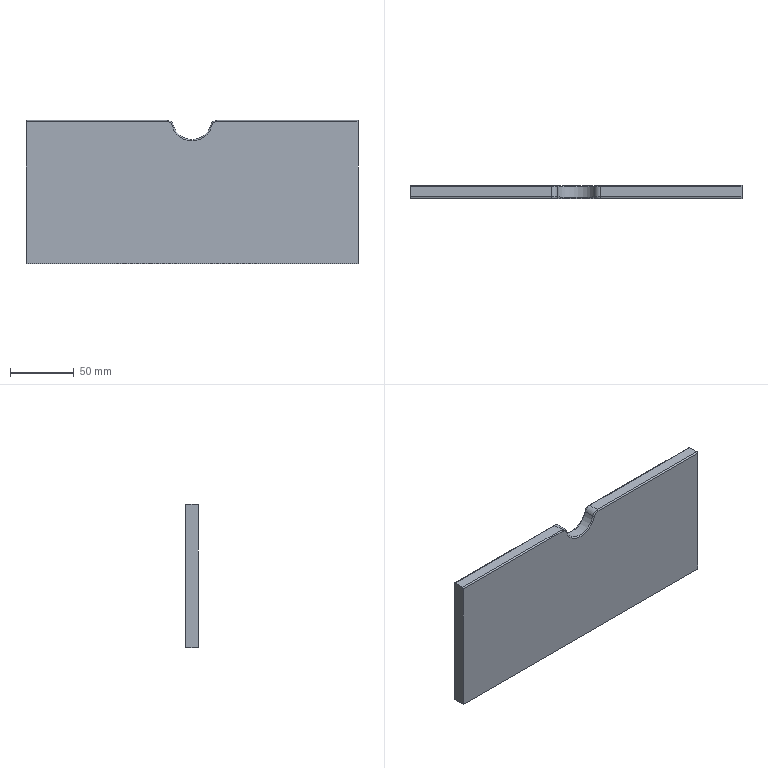Part | STEP file | Drawer | 1 solid | 20 faces | box 260 x 10 x 112 mm | volume 287478 mm3 | plane 7 | cylinder 7 | torus 6 | commonest cylinder face diameters 2 x4 10 x2 30 x1
STEP:
#1=CARTESIAN_POINT('',(0.,0.,0.));
#2=DIRECTION('',(0.,0.,1.));
#3=DIRECTION('',(1.,0.,0.));
#4=AXIS2_PLACEMENT_3D('',#1,#2,#3);
#5=CARTESIAN_POINT('',(-19.365,-9.,112.));
#6=VERTEX_POINT('',#5);
#7=CARTESIAN_POINT('',(-19.365,-1.,112.));
#8=VERTEX_POINT('',#7);
#9=CARTESIAN_POINT('',(-19.365,-10.,112.));
#10=DIRECTION('',(0.,1.,0.));
#11=VECTOR('',#10,1.);
#12=LINE('',#9,#11);
#13=CARTESIAN_POINT('',(130.,0.,112.));
#14=DIRECTION('',(0.,0.,-1.));
#15=DIRECTION('',(-1.,0.,0.));
#16=AXIS2_PLACEMENT_3D('',#13,#14,#15);
#17=PLANE('',#16);
#18=CARTESIAN_POINT('',(149.365,-10.));
#19=DIRECTION('',(0.,1.));
#20=VECTOR('',#19,1.);
#21=LINE('',#18,#20);
#22=(GEOMETRIC_REPRESENTATION_CONTEXT(2)PARAMETRIC_REPRESENTATION_CONTEXT()REPRESENTATION_CONTEXT('',''));
#23=DEFINITIONAL_REPRESENTATION('',(#21),#22);
#24=PCURVE('',#17,#23);
#25=CARTESIAN_POINT('',(-19.365,-10.,107.));
#26=DIRECTION('',(0.,1.,0.));
#27=DIRECTION('',(0.,0.,1.));
#28=AXIS2_PLACEMENT_3D('',#25,#26,#27);
#29=CYLINDRICAL_SURFACE('',#28,5.);
#30=CARTESIAN_POINT('',(0.,0.));
#31=DIRECTION('',(0.,1.));
#32=VECTOR('',#31,1.);
#33=LINE('',#30,#32);
#34=(GEOMETRIC_REPRESENTATION_CONTEXT(2)PARAMETRIC_REPRESENTATION_CONTEXT()REPRESENTATION_CONTEXT('',''));
#35=DEFINITIONAL_REPRESENTATION('',(#33),#34);
#36=PCURVE('',#29,#35);
#37=SURFACE_CURVE('',#12,(#24,#36),.PCURVE_S1.);
#38=EDGE_CURVE('',#6,#8,#37,.T.);
#39=ORIENTED_EDGE('',*,*,#38,.F.);
#40=CARTESIAN_POINT('',(-130.,-9.,112.));
#41=VERTEX_POINT('',#40);
#42=CARTESIAN_POINT('',(-130.,-9.,112.));
#43=DIRECTION('',(1.,0.,0.));
#44=VECTOR('',#43,1.);
#45=LINE('',#42,#44);
#46=CARTESIAN_POINT('',(260.,-9.));
#47=DIRECTION('',(-1.,0.));
#48=VECTOR('',#47,1.);
#49=LINE('',#46,#48);
#50=(GEOMETRIC_REPRESENTATION_CONTEXT(2)PARAMETRIC_REPRESENTATION_CONTEXT()REPRESENTATION_CONTEXT('',''));
#51=DEFINITIONAL_REPRESENTATION('',(#49),#50);
#52=PCURVE('',#17,#51);
#53=CARTESIAN_POINT('',(-130.,-9.,111.));
#54=DIRECTION('',(1.,0.,0.));
#55=DIRECTION('',(0.,-1.,0.));
#56=AXIS2_PLACEMENT_3D('',#53,#54,#55);
#57=CYLINDRICAL_SURFACE('',#56,1.);
#58=CARTESIAN_POINT('',(4.712,0.));
#59=DIRECTION('',(0.,1.));
#60=VECTOR('',#59,1.);
#61=LINE('',#58,#60);
#62=(GEOMETRIC_REPRESENTATION_CONTEXT(2)PARAMETRIC_REPRESENTATION_CONTEXT()REPRESENTATION_CONTEXT('',''));
#63=DEFINITIONAL_REPRESENTATION('',(#61),#62);
#64=PCURVE('',#57,#63);
#65=SURFACE_CURVE('',#45,(#52,#64),.PCURVE_S1.);
#66=EDGE_CURVE('',#41,#6,#65,.T.);
#67=ORIENTED_EDGE('',*,*,#66,.F.);
#68=CARTESIAN_POINT('',(-130.,-1.,112.));
#69=VERTEX_POINT('',#68);
#70=CARTESIAN_POINT('',(-130.,0.,112.));
#71=DIRECTION('',(0.,-1.,0.));
#72=VECTOR('',#71,1.);
#73=LINE('',#70,#72);
#74=CARTESIAN_POINT('',(260.,0.));
#75=DIRECTION('',(0.,-1.));
#76=VECTOR('',#75,1.);
#77=LINE('',#74,#76);
#78=(GEOMETRIC_REPRESENTATION_CONTEXT(2)PARAMETRIC_REPRESENTATION_CONTEXT()REPRESENTATION_CONTEXT('',''));
#79=DEFINITIONAL_REPRESENTATION('',(#77),#78);
#80=PCURVE('',#17,#79);
#81=CARTESIAN_POINT('',(-130.,0.,112.));
#82=DIRECTION('',(1.,0.,0.));
#83=DIRECTION('',(0.,0.,-1.));
#84=AXIS2_PLACEMENT_3D('',#81,#82,#83);
#85=PLANE('',#84);
#86=CARTESIAN_POINT('',(0.,0.));
#87=DIRECTION('',(0.,-1.));
#88=VECTOR('',#87,1.);
#89=LINE('',#86,#88);
#90=(GEOMETRIC_REPRESENTATION_CONTEXT(2)PARAMETRIC_REPRESENTATION_CONTEXT()REPRESENTATION_CONTEXT('',''));
#91=DEFINITIONAL_REPRESENTATION('',(#89),#90);
#92=PCURVE('',#85,#91);
#93=SURFACE_CURVE('',#73,(#80,#92),.PCURVE_S1.);
#94=EDGE_CURVE('',#69,#41,#93,.T.);
#95=ORIENTED_EDGE('',*,*,#94,.F.);
#96=CARTESIAN_POINT('',(-130.,-1.,112.));
#97=DIRECTION('',(1.,0.,0.));
#98=VECTOR('',#97,1.);
#99=LINE('',#96,#98);
#100=CARTESIAN_POINT('',(260.,-1.));
#101=DIRECTION('',(-1.,0.));
#102=VECTOR('',#101,1.);
#103=LINE('',#100,#102);
#104=(GEOMETRIC_REPRESENTATION_CONTEXT(2)PARAMETRIC_REPRESENTATION_CONTEXT()REPRESENTATION_CONTEXT('',''));
#105=DEFINITIONAL_REPRESENTATION('',(#103),#104);
#106=PCURVE('',#17,#105);
#107=CARTESIAN_POINT('',(-130.,-1.,111.));
#108=DIRECTION('',(1.,0.,0.));
#109=DIRECTION('',(0.,1.,0.));
#110=AXIS2_PLACEMENT_3D('',#107,#108,#109);
#111=CYLINDRICAL_SURFACE('',#110,1.);
#112=CARTESIAN_POINT('',(1.571,0.));
#113=DIRECTION('',(0.,1.));
#114=VECTOR('',#113,1.);
#115=LINE('',#112,#114);
#116=(GEOMETRIC_REPRESENTATION_CONTEXT(2)PARAMETRIC_REPRESENTATION_CONTEXT()REPRESENTATION_CONTEXT('',''));
#117=DEFINITIONAL_REPRESENTATION('',(#115),#116);
#118=PCURVE('',#111,#117);
#119=SURFACE_CURVE('',#99,(#106,#118),.PCURVE_S1.);
#120=EDGE_CURVE('',#69,#8,#119,.T.);
#121=ORIENTED_EDGE('',*,*,#120,.T.);
#122=EDGE_LOOP('',(#39,#67,#95,#121));
#123=FACE_BOUND('',#122,.F.);
#124=ADVANCED_FACE('',(#123),#17,.F.);
#125=ORIENTED_EDGE('',*,*,#38,.F.);
#126=CARTESIAN_POINT('',(-14.524,-9.,108.25));
#127=VERTEX_POINT('',#126);
#128=CARTESIAN_POINT('',(-19.365,-9.,107.));
#129=DIRECTION('',(0.,1.,0.));
#130=DIRECTION('',(0.,0.,1.));
#131=AXIS2_PLACEMENT_3D('',#128,#129,#130);
#132=CIRCLE('',#131,5.);
#133=CARTESIAN_POINT('',(0.,1.));
#134=DIRECTION('',(1.,0.));
#135=VECTOR('',#134,1.);
#136=LINE('',#133,#135);
#137=(GEOMETRIC_REPRESENTATION_CONTEXT(2)PARAMETRIC_REPRESENTATION_CONTEXT()REPRESENTATION_CONTEXT('',''));
#138=DEFINITIONAL_REPRESENTATION('',(#136),#137);
#139=PCURVE('',#29,#138);
#140=CARTESIAN_POINT('',(-19.365,-9.,107.));
#141=DIRECTION('',(0.,1.,0.));
#142=DIRECTION('',(0.,0.,1.));
#143=AXIS2_PLACEMENT_3D('',#140,#141,#142);
#144=TOROIDAL_SURFACE('',#143,4.,1.);
#145=CARTESIAN_POINT('',(0.,6.283));
#146=DIRECTION('',(1.,0.));
#147=VECTOR('',#146,1.);
#148=LINE('',#145,#147);
#149=(GEOMETRIC_REPRESENTATION_CONTEXT(2)PARAMETRIC_REPRESENTATION_CONTEXT()REPRESENTATION_CONTEXT('',''));
#150=DEFINITIONAL_REPRESENTATION('',(#148),#149);
#151=PCURVE('',#144,#150);
#152=SURFACE_CURVE('',#132,(#139,#151),.PCURVE_S1.);
#153=EDGE_CURVE('',#6,#127,#152,.T.);
#154=ORIENTED_EDGE('',*,*,#153,.T.);
#155=CARTESIAN_POINT('',(-14.524,-1.,108.25));
#156=VERTEX_POINT('',#155);
#157=CARTESIAN_POINT('',(-14.524,-10.,108.25));
#158=DIRECTION('',(0.,1.,0.));
#159=VECTOR('',#158,1.);
#160=LINE('',#157,#159);
#161=CARTESIAN_POINT('',(1.318,0.));
#162=DIRECTION('',(0.,1.));
#163=VECTOR('',#162,1.);
#164=LINE('',#161,#163);
#165=(GEOMETRIC_REPRESENTATION_CONTEXT(2)PARAMETRIC_REPRESENTATION_CONTEXT()REPRESENTATION_CONTEXT('',''));
#166=DEFINITIONAL_REPRESENTATION('',(#164),#165);
#167=PCURVE('',#29,#166);
#168=CARTESIAN_POINT('',(0.,0.,112.));
#169=DIRECTION('',(0.,1.,0.));
#170=DIRECTION('',(1.,0.,0.));
#171=AXIS2_PLACEMENT_3D('',#168,#169,#170);
#172=CYLINDRICAL_SURFACE('',#171,15.);
#173=CARTESIAN_POINT('',(2.889,-10.));
#174=DIRECTION('',(0.,1.));
#175=VECTOR('',#174,1.);
#176=LINE('',#173,#175);
#177=(GEOMETRIC_REPRESENTATION_CONTEXT(2)PARAMETRIC_REPRESENTATION_CONTEXT()REPRESENTATION_CONTEXT('',''));
#178=DEFINITIONAL_REPRESENTATION('',(#176),#177);
#179=PCURVE('',#172,#178);
#180=SURFACE_CURVE('',#160,(#167,#179),.PCURVE_S1.);
#181=EDGE_CURVE('',#127,#156,#180,.T.);
#182=ORIENTED_EDGE('',*,*,#181,.T.);
#183=CARTESIAN_POINT('',(-19.365,-1.,107.));
#184=DIRECTION('',(0.,1.,0.));
#185=DIRECTION('',(0.,0.,1.));
#186=AXIS2_PLACEMENT_3D('',#183,#184,#185);
#187=CIRCLE('',#186,5.);
#188=CARTESIAN_POINT('',(0.,9.));
#189=DIRECTION('',(1.,0.));
#190=VECTOR('',#189,1.);
#191=LINE('',#188,#190);
#192=(GEOMETRIC_REPRESENTATION_CONTEXT(2)PARAMETRIC_REPRESENTATION_CONTEXT()REPRESENTATION_CONTEXT('',''));
#193=DEFINITIONAL_REPRESENTATION('',(#191),#192);
#194=PCURVE('',#29,#193);
#195=CARTESIAN_POINT('',(-19.365,-1.,107.));
#196=DIRECTION('',(0.,-1.,0.));
#197=DIRECTION('',(0.,0.,1.));
#198=AXIS2_PLACEMENT_3D('',#195,#196,#197);
#199=TOROIDAL_SURFACE('',#198,4.,1.);
#200=CARTESIAN_POINT('',(6.283,6.283));
#201=DIRECTION('',(-1.,0.));
#202=VECTOR('',#201,1.);
#203=LINE('',#200,#202);
#204=(GEOMETRIC_REPRESENTATION_CONTEXT(2)PARAMETRIC_REPRESENTATION_CONTEXT()REPRESENTATION_CONTEXT('',''));
#205=DEFINITIONAL_REPRESENTATION('',(#203),#204);
#206=PCURVE('',#199,#205);
#207=SURFACE_CURVE('',#187,(#194,#206),.PCURVE_S1.);
#208=EDGE_CURVE('',#8,#156,#207,.T.);
#209=ORIENTED_EDGE('',*,*,#208,.F.);
#210=EDGE_LOOP('',(#125,#154,#182,#209));
#211=FACE_BOUND('',#210,.T.);
#212=ADVANCED_FACE('',(#211),#29,.T.);
#213=CARTESIAN_POINT('',(-130.,-10.,111.));
#214=VERTEX_POINT('',#213);
#215=CARTESIAN_POINT('',(-19.365,-10.,111.));
#216=VERTEX_POINT('',#215);
#217=CARTESIAN_POINT('',(-130.,-10.,111.));
#218=DIRECTION('',(1.,0.,0.));
#219=VECTOR('',#218,1.);
#220=LINE('',#217,#219);
#221=CARTESIAN_POINT('',(6.283,0.));
#222=DIRECTION('',(0.,1.));
#223=VECTOR('',#222,1.);
#224=LINE('',#221,#223);
#225=(GEOMETRIC_REPRESENTATION_CONTEXT(2)PARAMETRIC_REPRESENTATION_CONTEXT()REPRESENTATION_CONTEXT('',''));
#226=DEFINITIONAL_REPRESENTATION('',(#224),#225);
#227=PCURVE('',#57,#226);
#228=CARTESIAN_POINT('',(0.,-10.,56.));
#229=DIRECTION('',(0.,1.,0.));
#230=DIRECTION('',(0.,0.,1.));
#231=AXIS2_PLACEMENT_3D('',#228,#229,#230);
#232=PLANE('',#231);
#233=CARTESIAN_POINT('',(55.,-130.));
#234=DIRECTION('',(0.,1.));
#235=VECTOR('',#234,1.);
#236=LINE('',#233,#235);
#237=(GEOMETRIC_REPRESENTATION_CONTEXT(2)PARAMETRIC_REPRESENTATION_CONTEXT()REPRESENTATION_CONTEXT('',''));
#238=DEFINITIONAL_REPRESENTATION('',(#236),#237);
#239=PCURVE('',#232,#238);
#240=SURFACE_CURVE('',#220,(#227,#239),.PCURVE_S1.);
#241=EDGE_CURVE('',#214,#216,#240,.T.);
#242=ORIENTED_EDGE('',*,*,#241,.T.);
#243=CARTESIAN_POINT('',(-19.365,-9.,111.));
#244=DIRECTION('',(-1.,0.,0.));
#245=DIRECTION('',(0.,-1.,0.));
#246=AXIS2_PLACEMENT_3D('',#243,#244,#245);
#247=CIRCLE('',#246,1.);
#248=CARTESIAN_POINT('',(6.283,110.635));
#249=DIRECTION('',(-1.,0.));
#250=VECTOR('',#249,1.);
#251=LINE('',#248,#250);
#252=(GEOMETRIC_REPRESENTATION_CONTEXT(2)PARAMETRIC_REPRESENTATION_CONTEXT()REPRESENTATION_CONTEXT('',''));
#253=DEFINITIONAL_REPRESENTATION('',(#251),#252);
#254=PCURVE('',#57,#253);
#255=CARTESIAN_POINT('',(0.,4.712));
#256=DIRECTION('',(0.,1.));
#257=VECTOR('',#256,1.);
#258=LINE('',#255,#257);
#259=(GEOMETRIC_REPRESENTATION_CONTEXT(2)PARAMETRIC_REPRESENTATION_CONTEXT()REPRESENTATION_CONTEXT('',''));
#260=DEFINITIONAL_REPRESENTATION('',(#258),#259);
#261=PCURVE('',#144,#260);
#262=SURFACE_CURVE('',#247,(#254,#261),.PCURVE_S1.);
#263=EDGE_CURVE('',#216,#6,#262,.T.);
#264=ORIENTED_EDGE('',*,*,#263,.T.);
#265=ORIENTED_EDGE('',*,*,#66,.F.);
#266=CARTESIAN_POINT('',(-130.,-9.,111.));
#267=DIRECTION('',(-1.,0.,0.));
#268=DIRECTION('',(0.,0.,1.));
#269=AXIS2_PLACEMENT_3D('',#266,#267,#268);
#270=CIRCLE('',#269,1.);
#271=CARTESIAN_POINT('',(10.996,0.));
#272=DIRECTION('',(-1.,0.));
#273=VECTOR('',#272,1.);
#274=LINE('',#271,#273);
#275=(GEOMETRIC_REPRESENTATION_CONTEXT(2)PARAMETRIC_REPRESENTATION_CONTEXT()REPRESENTATION_CONTEXT('',''));
#276=DEFINITIONAL_REPRESENTATION('',(#274),#275);
#277=PCURVE('',#57,#276);
#278=CARTESIAN_POINT('',(0.,-9.));
#279=CARTESIAN_POINT('',(0.,-7.268));
#280=CARTESIAN_POINT('',(1.5,-8.134));
#281=CARTESIAN_POINT('',(3.,-9.));
#282=CARTESIAN_POINT('',(1.5,-9.866));
#283=CARTESIAN_POINT('',(0.,-10.732));
#284=CARTESIAN_POINT('',(0.,-9.));
#285=(BOUNDED_CURVE()B_SPLINE_CURVE(2,(#278,#279,#280,#281,#282,#283,#284),.UNSPECIFIED.,.T.,.F.)B_SPLINE_CURVE_WITH_KNOTS((1,2,2,2,2,1),(-2.094,0.,2.094,4.189,6.283,8.378),.UNSPECIFIED.)CURVE()GEOMETRIC_REPRESENTATION_ITEM()RATIONAL_B_SPLINE_CURVE((1.,0.5,1.,0.5,1.,0.5,1.))REPRESENTATION_ITEM(''));
#286=(GEOMETRIC_REPRESENTATION_CONTEXT(2)PARAMETRIC_REPRESENTATION_CONTEXT()REPRESENTATION_CONTEXT('',''));
#287=DEFINITIONAL_REPRESENTATION('',(#285),#286);
#288=PCURVE('',#85,#287);
#289=SURFACE_CURVE('',#270,(#277,#288),.PCURVE_S1.);
#290=EDGE_CURVE('',#214,#41,#289,.T.);
#291=ORIENTED_EDGE('',*,*,#290,.F.);
#292=EDGE_LOOP('',(#242,#264,#265,#291));
#293=FACE_BOUND('',#292,.T.);
#294=ADVANCED_FACE('',(#293),#57,.T.);
#295=CARTESIAN_POINT('',(-130.,0.,111.));
#296=VERTEX_POINT('',#295);
#297=CARTESIAN_POINT('',(-130.,-1.,111.));
#298=DIRECTION('',(1.,0.,0.));
#299=DIRECTION('',(0.,0.,1.));
#300=AXIS2_PLACEMENT_3D('',#297,#298,#299);
#301=CIRCLE('',#300,1.);
#302=CARTESIAN_POINT('',(-4.712,0.));
#303=DIRECTION('',(1.,0.));
#304=VECTOR('',#303,1.);
#305=LINE('',#302,#304);
#306=(GEOMETRIC_REPRESENTATION_CONTEXT(2)PARAMETRIC_REPRESENTATION_CONTEXT()REPRESENTATION_CONTEXT('',''));
#307=DEFINITIONAL_REPRESENTATION('',(#305),#306);
#308=PCURVE('',#111,#307);
#309=CARTESIAN_POINT('',(1.,-1.));
#310=DIRECTION('',(-1.,0.));
#311=AXIS2_PLACEMENT_2D('',#309,#310);
#312=CIRCLE('',#311,1.);
#313=(GEOMETRIC_REPRESENTATION_CONTEXT(2)PARAMETRIC_REPRESENTATION_CONTEXT()REPRESENTATION_CONTEXT('',''));
#314=DEFINITIONAL_REPRESENTATION('',(#312),#313);
#315=PCURVE('',#85,#314);
#316=SURFACE_CURVE('',#301,(#308,#315),.PCURVE_S1.);
#317=EDGE_CURVE('',#296,#69,#316,.T.);
#318=ORIENTED_EDGE('',*,*,#317,.T.);
#319=ORIENTED_EDGE('',*,*,#120,.T.);
#320=CARTESIAN_POINT('',(-19.365,0.,111.));
#321=VERTEX_POINT('',#320);
#322=CARTESIAN_POINT('',(-19.365,-1.,111.));
#323=DIRECTION('',(1.,0.,0.));
#324=DIRECTION('',(0.,1.,0.));
#325=AXIS2_PLACEMENT_3D('',#322,#323,#324);
#326=CIRCLE('',#325,1.);
#327=CARTESIAN_POINT('',(0.,110.635));
#328=DIRECTION('',(1.,0.));
#329=VECTOR('',#328,1.);
#330=LINE('',#327,#329);
#331=(GEOMETRIC_REPRESENTATION_CONTEXT(2)PARAMETRIC_REPRESENTATION_CONTEXT()REPRESENTATION_CONTEXT('',''));
#332=DEFINITIONAL_REPRESENTATION('',(#330),#331);
#333=PCURVE('',#111,#332);
#334=CARTESIAN_POINT('',(6.283,4.712));
#335=DIRECTION('',(0.,1.));
#336=VECTOR('',#335,1.);
#337=LINE('',#334,#336);
#338=(GEOMETRIC_REPRESENTATION_CONTEXT(2)PARAMETRIC_REPRESENTATION_CONTEXT()REPRESENTATION_CONTEXT('',''));
#339=DEFINITIONAL_REPRESENTATION('',(#337),#338);
#340=PCURVE('',#199,#339);
#341=SURFACE_CURVE('',#326,(#333,#340),.PCURVE_S1.);
#342=EDGE_CURVE('',#321,#8,#341,.T.);
#343=ORIENTED_EDGE('',*,*,#342,.F.);
#344=CARTESIAN_POINT('',(-130.,0.,111.));
#345=DIRECTION('',(1.,0.,0.));
#346=VECTOR('',#345,1.);
#347=LINE('',#344,#346);
#348=CARTESIAN_POINT('',(0.,0.));
#349=DIRECTION('',(0.,1.));
#350=VECTOR('',#349,1.);
#351=LINE('',#348,#350);
#352=(GEOMETRIC_REPRESENTATION_CONTEXT(2)PARAMETRIC_REPRESENTATION_CONTEXT()REPRESENTATION_CONTEXT('',''));
#353=DEFINITIONAL_REPRESENTATION('',(#351),#352);
#354=PCURVE('',#111,#353);
#355=CARTESIAN_POINT('',(0.,0.,56.));
#356=DIRECTION('',(0.,1.,0.));
#357=DIRECTION('',(0.,0.,1.));
#358=AXIS2_PLACEMENT_3D('',#355,#356,#357);
#359=PLANE('',#358);
#360=CARTESIAN_POINT('',(55.,-130.));
#361=DIRECTION('',(0.,1.));
#362=VECTOR('',#361,1.);
#363=LINE('',#360,#362);
#364=(GEOMETRIC_REPRESENTATION_CONTEXT(2)PARAMETRIC_REPRESENTATION_CONTEXT()REPRESENTATION_CONTEXT('',''));
#365=DEFINITIONAL_REPRESENTATION('',(#363),#364);
#366=PCURVE('',#359,#365);
#367=SURFACE_CURVE('',#347,(#354,#366),.PCURVE_S1.);
#368=EDGE_CURVE('',#296,#321,#367,.T.);
#369=ORIENTED_EDGE('',*,*,#368,.F.);
#370=EDGE_LOOP('',(#318,#319,#343,#369));
#371=FACE_BOUND('',#370,.T.);
#372=ADVANCED_FACE('',(#371),#111,.T.);
#373=ORIENTED_EDGE('',*,*,#94,.T.);
#374=ORIENTED_EDGE('',*,*,#290,.F.);
#375=CARTESIAN_POINT('',(-130.,-10.,0.));
#376=VERTEX_POINT('',#375);
#377=CARTESIAN_POINT('',(-130.,-10.,112.));
#378=DIRECTION('',(0.,0.,-1.));
#379=VECTOR('',#378,1.);
#380=LINE('',#377,#379);
#381=CARTESIAN_POINT('',(0.,-10.));
#382=DIRECTION('',(1.,0.));
#383=VECTOR('',#382,1.);
#384=LINE('',#381,#383);
#385=(GEOMETRIC_REPRESENTATION_CONTEXT(2)PARAMETRIC_REPRESENTATION_CONTEXT()REPRESENTATION_CONTEXT('',''));
#386=DEFINITIONAL_REPRESENTATION('',(#384),#385);
#387=PCURVE('',#85,#386);
#388=CARTESIAN_POINT('',(56.,-130.));
#389=DIRECTION('',(-1.,0.));
#390=VECTOR('',#389,1.);
#391=LINE('',#388,#390);
#392=(GEOMETRIC_REPRESENTATION_CONTEXT(2)PARAMETRIC_REPRESENTATION_CONTEXT()REPRESENTATION_CONTEXT('',''));
#393=DEFINITIONAL_REPRESENTATION('',(#391),#392);
#394=PCURVE('',#232,#393);
#395=SURFACE_CURVE('',#380,(#387,#394),.PCURVE_S1.);
#396=EDGE_CURVE('',#214,#376,#395,.T.);
#397=ORIENTED_EDGE('',*,*,#396,.T.);
#398=CARTESIAN_POINT('',(-130.,0.,0.));
#399=VERTEX_POINT('',#398);
#400=CARTESIAN_POINT('',(-130.,0.,0.));
#401=DIRECTION('',(0.,-1.,0.));
#402=VECTOR('',#401,1.);
#403=LINE('',#400,#402);
#404=CARTESIAN_POINT('',(112.,0.));
#405=DIRECTION('',(0.,-1.));
#406=VECTOR('',#405,1.);
#407=LINE('',#404,#406);
#408=(GEOMETRIC_REPRESENTATION_CONTEXT(2)PARAMETRIC_REPRESENTATION_CONTEXT()REPRESENTATION_CONTEXT('',''));
#409=DEFINITIONAL_REPRESENTATION('',(#407),#408);
#410=PCURVE('',#85,#409);
#411=CARTESIAN_POINT('',(-130.,0.,0.));
#412=DIRECTION('',(0.,0.,1.));
#413=DIRECTION('',(1.,0.,0.));
#414=AXIS2_PLACEMENT_3D('',#411,#412,#413);
#415=PLANE('',#414);
#416=CARTESIAN_POINT('',(0.,0.));
#417=DIRECTION('',(0.,-1.));
#418=VECTOR('',#417,1.);
#419=LINE('',#416,#418);
#420=(GEOMETRIC_REPRESENTATION_CONTEXT(2)PARAMETRIC_REPRESENTATION_CONTEXT()REPRESENTATION_CONTEXT('',''));
#421=DEFINITIONAL_REPRESENTATION('',(#419),#420);
#422=PCURVE('',#415,#421);
#423=SURFACE_CURVE('',#403,(#410,#422),.PCURVE_S1.);
#424=EDGE_CURVE('',#399,#376,#423,.T.);
#425=ORIENTED_EDGE('',*,*,#424,.F.);
#426=CARTESIAN_POINT('',(-130.,0.,112.));
#427=DIRECTION('',(0.,0.,-1.));
#428=VECTOR('',#427,1.);
#429=LINE('',#426,#428);
#430=CARTESIAN_POINT('',(0.,0.));
#431=DIRECTION('',(1.,0.));
#432=VECTOR('',#431,1.);
#433=LINE('',#430,#432);
#434=(GEOMETRIC_REPRESENTATION_CONTEXT(2)PARAMETRIC_REPRESENTATION_CONTEXT()REPRESENTATION_CONTEXT('',''));
#435=DEFINITIONAL_REPRESENTATION('',(#433),#434);
#436=PCURVE('',#85,#435);
#437=CARTESIAN_POINT('',(56.,-130.));
#438=DIRECTION('',(-1.,0.));
#439=VECTOR('',#438,1.);
#440=LINE('',#437,#439);
#441=(GEOMETRIC_REPRESENTATION_CONTEXT(2)PARAMETRIC_REPRESENTATION_CONTEXT()REPRESENTATION_CONTEXT('',''));
#442=DEFINITIONAL_REPRESENTATION('',(#440),#441);
#443=PCURVE('',#359,#442);
#444=SURFACE_CURVE('',#429,(#436,#443),.PCURVE_S1.);
#445=EDGE_CURVE('',#296,#399,#444,.T.);
#446=ORIENTED_EDGE('',*,*,#445,.F.);
#447=ORIENTED_EDGE('',*,*,#317,.T.);
#448=EDGE_LOOP('',(#373,#374,#397,#425,#446,#447));
#449=FACE_BOUND('',#448,.F.);
#450=ADVANCED_FACE('',(#449),#85,.F.);
#451=ORIENTED_EDGE('',*,*,#263,.F.);
#452=CARTESIAN_POINT('',(-15.492,-10.,108.));
#453=VERTEX_POINT('',#452);
#454=CARTESIAN_POINT('',(-19.365,-10.,107.));
#455=DIRECTION('',(0.,1.,0.));
#456=DIRECTION('',(0.,0.,1.));
#457=AXIS2_PLACEMENT_3D('',#454,#455,#456);
#458=CIRCLE('',#457,4.);
#459=CARTESIAN_POINT('',(0.,4.712));
#460=DIRECTION('',(1.,0.));
#461=VECTOR('',#460,1.);
#462=LINE('',#459,#461);
#463=(GEOMETRIC_REPRESENTATION_CONTEXT(2)PARAMETRIC_REPRESENTATION_CONTEXT()REPRESENTATION_CONTEXT('',''));
#464=DEFINITIONAL_REPRESENTATION('',(#462),#463);
#465=PCURVE('',#144,#464);
#466=CARTESIAN_POINT('',(51.,-19.365));
#467=DIRECTION('',(1.,0.));
#468=AXIS2_PLACEMENT_2D('',#466,#467);
#469=CIRCLE('',#468,4.);
#470=(GEOMETRIC_REPRESENTATION_CONTEXT(2)PARAMETRIC_REPRESENTATION_CONTEXT()REPRESENTATION_CONTEXT('',''));
#471=DEFINITIONAL_REPRESENTATION('',(#469),#470);
#472=PCURVE('',#232,#471);
#473=SURFACE_CURVE('',#458,(#465,#472),.PCURVE_S1.);
#474=EDGE_CURVE('',#216,#453,#473,.T.);
#475=ORIENTED_EDGE('',*,*,#474,.T.);
#476=CARTESIAN_POINT('',(-15.492,-9.,108.));
#477=DIRECTION('',(-0.25,0.,0.9682));
#478=DIRECTION('',(0.9682,0.,0.25));
#479=AXIS2_PLACEMENT_3D('',#476,#477,#478);
#480=CIRCLE('',#479,1.);
#481=CARTESIAN_POINT('',(1.318,0.));
#482=DIRECTION('',(0.,1.));
#483=VECTOR('',#482,1.);
#484=LINE('',#481,#483);
#485=(GEOMETRIC_REPRESENTATION_CONTEXT(2)PARAMETRIC_REPRESENTATION_CONTEXT()REPRESENTATION_CONTEXT('',''));
#486=DEFINITIONAL_REPRESENTATION('',(#484),#485);
#487=PCURVE('',#144,#486);
#488=CARTESIAN_POINT('',(0.,-9.,112.));
#489=DIRECTION('',(0.,-1.,0.));
#490=DIRECTION('',(-0.9682,0.,-0.25));
#491=AXIS2_PLACEMENT_3D('',#488,#489,#490);
#492=TOROIDAL_SURFACE('',#491,16.,1.);
#493=CARTESIAN_POINT('',(0.,-3.142));
#494=DIRECTION('',(0.,1.));
#495=VECTOR('',#494,1.);
#496=LINE('',#493,#495);
#497=(GEOMETRIC_REPRESENTATION_CONTEXT(2)PARAMETRIC_REPRESENTATION_CONTEXT()REPRESENTATION_CONTEXT('',''));
#498=DEFINITIONAL_REPRESENTATION('',(#496),#497);
#499=PCURVE('',#492,#498);
#500=SURFACE_CURVE('',#480,(#487,#499),.PCURVE_S1.);
#501=EDGE_CURVE('',#453,#127,#500,.T.);
#502=ORIENTED_EDGE('',*,*,#501,.T.);
#503=ORIENTED_EDGE('',*,*,#153,.F.);
#504=EDGE_LOOP('',(#451,#475,#502,#503));
#505=FACE_BOUND('',#504,.T.);
#506=ADVANCED_FACE('',(#505),#144,.T.);
#507=ORIENTED_EDGE('',*,*,#208,.T.);
#508=CARTESIAN_POINT('',(-15.492,0.,108.));
#509=VERTEX_POINT('',#508);
#510=CARTESIAN_POINT('',(-15.492,-1.,108.));
#511=DIRECTION('',(0.25,0.,-0.9682));
#512=DIRECTION('',(0.9682,0.,0.25));
#513=AXIS2_PLACEMENT_3D('',#510,#511,#512);
#514=CIRCLE('',#513,1.);
#515=CARTESIAN_POINT('',(4.965,0.));
#516=DIRECTION('',(0.,1.));
#517=VECTOR('',#516,1.);
#518=LINE('',#515,#517);
#519=(GEOMETRIC_REPRESENTATION_CONTEXT(2)PARAMETRIC_REPRESENTATION_CONTEXT()REPRESENTATION_CONTEXT('',''));
#520=DEFINITIONAL_REPRESENTATION('',(#518),#519);
#521=PCURVE('',#199,#520);
#522=CARTESIAN_POINT('',(0.,-1.,112.));
#523=DIRECTION('',(0.,1.,0.));
#524=DIRECTION('',(-0.9682,0.,-0.25));
#525=AXIS2_PLACEMENT_3D('',#522,#523,#524);
#526=TOROIDAL_SURFACE('',#525,16.,1.);
#527=CARTESIAN_POINT('',(6.283,-3.142));
#528=DIRECTION('',(0.,1.));
#529=VECTOR('',#528,1.);
#530=LINE('',#527,#529);
#531=(GEOMETRIC_REPRESENTATION_CONTEXT(2)PARAMETRIC_REPRESENTATION_CONTEXT()REPRESENTATION_CONTEXT('',''));
#532=DEFINITIONAL_REPRESENTATION('',(#530),#531);
#533=PCURVE('',#526,#532);
#534=SURFACE_CURVE('',#514,(#521,#533),.PCURVE_S1.);
#535=EDGE_CURVE('',#509,#156,#534,.T.);
#536=ORIENTED_EDGE('',*,*,#535,.F.);
#537=CARTESIAN_POINT('',(-19.365,0.,107.));
#538=DIRECTION('',(0.,1.,0.));
#539=DIRECTION('',(0.,0.,1.));
#540=AXIS2_PLACEMENT_3D('',#537,#538,#539);
#541=CIRCLE('',#540,4.);
#542=CARTESIAN_POINT('',(6.283,4.712));
#543=DIRECTION('',(-1.,0.));
#544=VECTOR('',#543,1.);
#545=LINE('',#542,#544);
#546=(GEOMETRIC_REPRESENTATION_CONTEXT(2)PARAMETRIC_REPRESENTATION_CONTEXT()REPRESENTATION_CONTEXT('',''));
#547=DEFINITIONAL_REPRESENTATION('',(#545),#546);
#548=PCURVE('',#199,#547);
#549=CARTESIAN_POINT('',(51.,-19.365));
#550=DIRECTION('',(1.,0.));
#551=AXIS2_PLACEMENT_2D('',#549,#550);
#552=CIRCLE('',#551,4.);
#553=(GEOMETRIC_REPRESENTATION_CONTEXT(2)PARAMETRIC_REPRESENTATION_CONTEXT()REPRESENTATION_CONTEXT('',''));
#554=DEFINITIONAL_REPRESENTATION('',(#552),#553);
#555=PCURVE('',#359,#554);
#556=SURFACE_CURVE('',#541,(#548,#555),.PCURVE_S1.);
#557=EDGE_CURVE('',#321,#509,#556,.T.);
#558=ORIENTED_EDGE('',*,*,#557,.F.);
#559=ORIENTED_EDGE('',*,*,#342,.T.);
#560=EDGE_LOOP('',(#507,#536,#558,#559));
#561=FACE_BOUND('',#560,.T.);
#562=ADVANCED_FACE('',(#561),#199,.T.);
#563=CARTESIAN_POINT('',(14.524,-1.,108.25));
#564=VERTEX_POINT('',#563);
#565=CARTESIAN_POINT('',(0.,-1.,112.));
#566=DIRECTION('',(0.,-1.,0.));
#567=DIRECTION('',(-0.9682,0.,-0.25));
#568=AXIS2_PLACEMENT_3D('',#565,#566,#567);
#569=CIRCLE('',#568,15.);
#570=CARTESIAN_POINT('',(2.889,-1.));
#571=DIRECTION('',(-1.,0.));
#572=VECTOR('',#571,1.);
#573=LINE('',#570,#572);
#574=(GEOMETRIC_REPRESENTATION_CONTEXT(2)PARAMETRIC_REPRESENTATION_CONTEXT()REPRESENTATION_CONTEXT('',''));
#575=DEFINITIONAL_REPRESENTATION('',(#573),#574);
#576=PCURVE('',#172,#575);
#577=CARTESIAN_POINT('',(6.283,3.142));
#578=DIRECTION('',(-1.,0.));
#579=VECTOR('',#578,1.);
#580=LINE('',#577,#579);
#581=(GEOMETRIC_REPRESENTATION_CONTEXT(2)PARAMETRIC_REPRESENTATION_CONTEXT()REPRESENTATION_CONTEXT('',''));
#582=DEFINITIONAL_REPRESENTATION('',(#580),#581);
#583=PCURVE('',#526,#582);
#584=SURFACE_CURVE('',#569,(#576,#583),.PCURVE_S1.);
#585=EDGE_CURVE('',#156,#564,#584,.T.);
#586=ORIENTED_EDGE('',*,*,#585,.T.);
#587=CARTESIAN_POINT('',(14.524,-9.,108.25));
#588=VERTEX_POINT('',#587);
#589=CARTESIAN_POINT('',(14.524,0.,108.25));
#590=DIRECTION('',(0.,-1.,0.));
#591=VECTOR('',#590,1.);
#592=LINE('',#589,#591);
#593=CARTESIAN_POINT('',(0.2527,0.));
#594=DIRECTION('',(0.,-1.));
#595=VECTOR('',#594,1.);
#596=LINE('',#593,#595);
#597=(GEOMETRIC_REPRESENTATION_CONTEXT(2)PARAMETRIC_REPRESENTATION_CONTEXT()REPRESENTATION_CONTEXT('',''));
#598=DEFINITIONAL_REPRESENTATION('',(#596),#597);
#599=PCURVE('',#172,#598);
#600=CARTESIAN_POINT('',(19.365,0.,107.));
#601=DIRECTION('',(0.,-1.,0.));
#602=DIRECTION('',(-0.9682,0.,0.25));
#603=AXIS2_PLACEMENT_3D('',#600,#601,#602);
#604=CYLINDRICAL_SURFACE('',#603,5.);
#605=CARTESIAN_POINT('',(6.283,0.));
#606=DIRECTION('',(0.,1.));
#607=VECTOR('',#606,1.);
#608=LINE('',#605,#607);
#609=(GEOMETRIC_REPRESENTATION_CONTEXT(2)PARAMETRIC_REPRESENTATION_CONTEXT()REPRESENTATION_CONTEXT('',''));
#610=DEFINITIONAL_REPRESENTATION('',(#608),#609);
#611=PCURVE('',#604,#610);
#612=SURFACE_CURVE('',#592,(#599,#611),.PCURVE_S1.);
#613=EDGE_CURVE('',#564,#588,#612,.T.);
#614=ORIENTED_EDGE('',*,*,#613,.T.);
#615=CARTESIAN_POINT('',(0.,-9.,112.));
#616=DIRECTION('',(0.,-1.,0.));
#617=DIRECTION('',(-0.9682,0.,-0.25));
#618=AXIS2_PLACEMENT_3D('',#615,#616,#617);
#619=CIRCLE('',#618,15.);
#620=CARTESIAN_POINT('',(2.889,-9.));
#621=DIRECTION('',(-1.,0.));
#622=VECTOR('',#621,1.);
#623=LINE('',#620,#622);
#624=(GEOMETRIC_REPRESENTATION_CONTEXT(2)PARAMETRIC_REPRESENTATION_CONTEXT()REPRESENTATION_CONTEXT('',''));
#625=DEFINITIONAL_REPRESENTATION('',(#623),#624);
#626=PCURVE('',#172,#625);
#627=CARTESIAN_POINT('',(0.,3.142));
#628=DIRECTION('',(1.,0.));
#629=VECTOR('',#628,1.);
#630=LINE('',#627,#629);
#631=(GEOMETRIC_REPRESENTATION_CONTEXT(2)PARAMETRIC_REPRESENTATION_CONTEXT()REPRESENTATION_CONTEXT('',''));
#632=DEFINITIONAL_REPRESENTATION('',(#630),#631);
#633=PCURVE('',#492,#632);
#634=SURFACE_CURVE('',#619,(#626,#633),.PCURVE_S1.);
#635=EDGE_CURVE('',#127,#588,#634,.T.);
#636=ORIENTED_EDGE('',*,*,#635,.F.);
#637=ORIENTED_EDGE('',*,*,#181,.T.);
#638=EDGE_LOOP('',(#586,#614,#636,#637));
#639=FACE_BOUND('',#638,.F.);
#640=ADVANCED_FACE('',(#639),#172,.F.);
#641=CARTESIAN_POINT('',(130.,-10.,0.));
#642=VERTEX_POINT('',#641);
#643=CARTESIAN_POINT('',(130.,-10.,111.));
#644=VERTEX_POINT('',#643);
#645=CARTESIAN_POINT('',(130.,-10.,0.));
#646=DIRECTION('',(0.,0.,1.));
#647=VECTOR('',#646,1.);
#648=LINE('',#645,#647);
#649=CARTESIAN_POINT('',(-56.,130.));
#650=DIRECTION('',(1.,0.));
#651=VECTOR('',#650,1.);
#652=LINE('',#649,#651);
#653=(GEOMETRIC_REPRESENTATION_CONTEXT(2)PARAMETRIC_REPRESENTATION_CONTEXT()REPRESENTATION_CONTEXT('',''));
#654=DEFINITIONAL_REPRESENTATION('',(#652),#653);
#655=PCURVE('',#232,#654);
#656=CARTESIAN_POINT('',(130.,0.,0.));
#657=DIRECTION('',(-1.,0.,0.));
#658=DIRECTION('',(0.,0.,1.));
#659=AXIS2_PLACEMENT_3D('',#656,#657,#658);
#660=PLANE('',#659);
#661=CARTESIAN_POINT('',(0.,-10.));
#662=DIRECTION('',(1.,0.));
#663=VECTOR('',#662,1.);
#664=LINE('',#661,#663);
#665=(GEOMETRIC_REPRESENTATION_CONTEXT(2)PARAMETRIC_REPRESENTATION_CONTEXT()REPRESENTATION_CONTEXT('',''));
#666=DEFINITIONAL_REPRESENTATION('',(#664),#665);
#667=PCURVE('',#660,#666);
#668=SURFACE_CURVE('',#648,(#655,#667),.PCURVE_S1.);
#669=EDGE_CURVE('',#642,#644,#668,.T.);
#670=ORIENTED_EDGE('',*,*,#669,.F.);
#671=CARTESIAN_POINT('',(-130.,-10.,0.));
#672=DIRECTION('',(1.,0.,0.));
#673=VECTOR('',#672,1.);
#674=LINE('',#671,#673);
#675=CARTESIAN_POINT('',(-56.,-130.));
#676=DIRECTION('',(0.,1.));
#677=VECTOR('',#676,1.);
#678=LINE('',#675,#677);
#679=(GEOMETRIC_REPRESENTATION_CONTEXT(2)PARAMETRIC_REPRESENTATION_CONTEXT()REPRESENTATION_CONTEXT('',''));
#680=DEFINITIONAL_REPRESENTATION('',(#678),#679);
#681=PCURVE('',#232,#680);
#682=CARTESIAN_POINT('',(0.,-10.));
#683=DIRECTION('',(1.,0.));
#684=VECTOR('',#683,1.);
#685=LINE('',#682,#684);
#686=(GEOMETRIC_REPRESENTATION_CONTEXT(2)PARAMETRIC_REPRESENTATION_CONTEXT()REPRESENTATION_CONTEXT('',''));
#687=DEFINITIONAL_REPRESENTATION('',(#685),#686);
#688=PCURVE('',#415,#687);
#689=SURFACE_CURVE('',#674,(#681,#688),.PCURVE_S1.);
#690=EDGE_CURVE('',#376,#642,#689,.T.);
#691=ORIENTED_EDGE('',*,*,#690,.F.);
#692=ORIENTED_EDGE('',*,*,#396,.F.);
#693=ORIENTED_EDGE('',*,*,#241,.T.);
#694=ORIENTED_EDGE('',*,*,#474,.T.);
#695=CARTESIAN_POINT('',(15.492,-10.,108.));
#696=VERTEX_POINT('',#695);
#697=CARTESIAN_POINT('',(0.,-10.,112.));
#698=DIRECTION('',(0.,-1.,0.));
#699=DIRECTION('',(-0.9682,0.,-0.25));
#700=AXIS2_PLACEMENT_3D('',#697,#698,#699);
#701=CIRCLE('',#700,16.);
#702=CARTESIAN_POINT('',(52.,-15.492));
#703=CARTESIAN_POINT('',(25.167,-8.564));
#704=CARTESIAN_POINT('',(44.584,11.21));
#705=CARTESIAN_POINT('',(64.,30.984));
#706=CARTESIAN_POINT('',(71.416,4.282));
#707=CARTESIAN_POINT('',(78.833,-22.42));
#708=CARTESIAN_POINT('',(52.,-15.492));
#709=(BOUNDED_CURVE()B_SPLINE_CURVE(2,(#702,#703,#704,#705,#706,#707,#708),.UNSPECIFIED.,.T.,.F.)B_SPLINE_CURVE_WITH_KNOTS((1,2,2,2,2,1),(-2.094,0.,2.094,4.189,6.283,8.378),.UNSPECIFIED.)CURVE()GEOMETRIC_REPRESENTATION_ITEM()RATIONAL_B_SPLINE_CURVE((1.,0.5,1.,0.5,1.,0.5,1.))REPRESENTATION_ITEM(''));
#710=(GEOMETRIC_REPRESENTATION_CONTEXT(2)PARAMETRIC_REPRESENTATION_CONTEXT()REPRESENTATION_CONTEXT('',''));
#711=DEFINITIONAL_REPRESENTATION('',(#709),#710);
#712=PCURVE('',#232,#711);
#713=CARTESIAN_POINT('',(0.,1.571));
#714=DIRECTION('',(1.,0.));
#715=VECTOR('',#714,1.);
#716=LINE('',#713,#715);
#717=(GEOMETRIC_REPRESENTATION_CONTEXT(2)PARAMETRIC_REPRESENTATION_CONTEXT()REPRESENTATION_CONTEXT('',''));
#718=DEFINITIONAL_REPRESENTATION('',(#716),#717);
#719=PCURVE('',#492,#718);
#720=SURFACE_CURVE('',#701,(#712,#719),.PCURVE_S1.);
#721=EDGE_CURVE('',#453,#696,#720,.T.);
#722=ORIENTED_EDGE('',*,*,#721,.T.);
#723=CARTESIAN_POINT('',(19.365,-10.,111.));
#724=VERTEX_POINT('',#723);
#725=CARTESIAN_POINT('',(19.365,-10.,107.));
#726=DIRECTION('',(0.,1.,0.));
#727=DIRECTION('',(-0.9682,0.,0.25));
#728=AXIS2_PLACEMENT_3D('',#725,#726,#727);
#729=CIRCLE('',#728,4.);
#730=CARTESIAN_POINT('',(51.,19.365));
#731=DIRECTION('',(0.25,-0.9682));
#732=AXIS2_PLACEMENT_2D('',#730,#731);
#733=CIRCLE('',#732,4.);
#734=(GEOMETRIC_REPRESENTATION_CONTEXT(2)PARAMETRIC_REPRESENTATION_CONTEXT()REPRESENTATION_CONTEXT('',''));
#735=DEFINITIONAL_REPRESENTATION('',(#733),#734);
#736=PCURVE('',#232,#735);
#737=CARTESIAN_POINT('',(19.365,-9.,107.));
#738=DIRECTION('',(0.,1.,0.));
#739=DIRECTION('',(-0.9682,0.,0.25));
#740=AXIS2_PLACEMENT_3D('',#737,#738,#739);
#741=TOROIDAL_SURFACE('',#740,4.,1.);
#742=CARTESIAN_POINT('',(0.,4.712));
#743=DIRECTION('',(1.,0.));
#744=VECTOR('',#743,1.);
#745=LINE('',#742,#744);
#746=(GEOMETRIC_REPRESENTATION_CONTEXT(2)PARAMETRIC_REPRESENTATION_CONTEXT()REPRESENTATION_CONTEXT('',''));
#747=DEFINITIONAL_REPRESENTATION('',(#745),#746);
#748=PCURVE('',#741,#747);
#749=SURFACE_CURVE('',#729,(#736,#748),.PCURVE_S1.);
#750=EDGE_CURVE('',#696,#724,#749,.T.);
#751=ORIENTED_EDGE('',*,*,#750,.T.);
#752=CARTESIAN_POINT('',(19.365,-10.,111.));
#753=DIRECTION('',(1.,0.,0.));
#754=VECTOR('',#753,1.);
#755=LINE('',#752,#754);
#756=CARTESIAN_POINT('',(55.,19.365));
#757=DIRECTION('',(0.,1.));
#758=VECTOR('',#757,1.);
#759=LINE('',#756,#758);
#760=(GEOMETRIC_REPRESENTATION_CONTEXT(2)PARAMETRIC_REPRESENTATION_CONTEXT()REPRESENTATION_CONTEXT('',''));
#761=DEFINITIONAL_REPRESENTATION('',(#759),#760);
#762=PCURVE('',#232,#761);
#763=CARTESIAN_POINT('',(19.365,-9.,111.));
#764=DIRECTION('',(1.,0.,0.));
#765=DIRECTION('',(0.,-1.,0.));
#766=AXIS2_PLACEMENT_3D('',#763,#764,#765);
#767=CYLINDRICAL_SURFACE('',#766,1.);
#768=CARTESIAN_POINT('',(6.283,0.));
#769=DIRECTION('',(0.,1.));
#770=VECTOR('',#769,1.);
#771=LINE('',#768,#770);
#772=(GEOMETRIC_REPRESENTATION_CONTEXT(2)PARAMETRIC_REPRESENTATION_CONTEXT()REPRESENTATION_CONTEXT('',''));
#773=DEFINITIONAL_REPRESENTATION('',(#771),#772);
#774=PCURVE('',#767,#773);
#775=SURFACE_CURVE('',#755,(#762,#774),.PCURVE_S1.);
#776=EDGE_CURVE('',#724,#644,#775,.T.);
#777=ORIENTED_EDGE('',*,*,#776,.T.);
#778=EDGE_LOOP('',(#670,#691,#692,#693,#694,#722,#751,#777));
#779=FACE_BOUND('',#778,.F.);
#780=ADVANCED_FACE('',(#779),#232,.F.);
#781=CARTESIAN_POINT('',(130.,0.,0.));
#782=VERTEX_POINT('',#781);
#783=CARTESIAN_POINT('',(130.,0.,111.));
#784=VERTEX_POINT('',#783);
#785=CARTESIAN_POINT('',(130.,0.,0.));
#786=DIRECTION('',(0.,0.,1.));
#787=VECTOR('',#786,1.);
#788=LINE('',#785,#787);
#789=CARTESIAN_POINT('',(-56.,130.));
#790=DIRECTION('',(1.,0.));
#791=VECTOR('',#790,1.);
#792=LINE('',#789,#791);
#793=(GEOMETRIC_REPRESENTATION_CONTEXT(2)PARAMETRIC_REPRESENTATION_CONTEXT()REPRESENTATION_CONTEXT('',''));
#794=DEFINITIONAL_REPRESENTATION('',(#792),#793);
#795=PCURVE('',#359,#794);
#796=CARTESIAN_POINT('',(0.,0.));
#797=DIRECTION('',(1.,0.));
#798=VECTOR('',#797,1.);
#799=LINE('',#796,#798);
#800=(GEOMETRIC_REPRESENTATION_CONTEXT(2)PARAMETRIC_REPRESENTATION_CONTEXT()REPRESENTATION_CONTEXT('',''));
#801=DEFINITIONAL_REPRESENTATION('',(#799),#800);
#802=PCURVE('',#660,#801);
#803=SURFACE_CURVE('',#788,(#795,#802),.PCURVE_S1.);
#804=EDGE_CURVE('',#782,#784,#803,.T.);
#805=ORIENTED_EDGE('',*,*,#804,.F.);
#806=CARTESIAN_POINT('',(-130.,0.,0.));
#807=DIRECTION('',(1.,0.,0.));
#808=VECTOR('',#807,1.);
#809=LINE('',#806,#808);
#810=CARTESIAN_POINT('',(-56.,-130.));
#811=DIRECTION('',(0.,1.));
#812=VECTOR('',#811,1.);
#813=LINE('',#810,#812);
#814=(GEOMETRIC_REPRESENTATION_CONTEXT(2)PARAMETRIC_REPRESENTATION_CONTEXT()REPRESENTATION_CONTEXT('',''));
#815=DEFINITIONAL_REPRESENTATION('',(#813),#814);
#816=PCURVE('',#359,#815);
#817=CARTESIAN_POINT('',(0.,0.));
#818=DIRECTION('',(1.,0.));
#819=VECTOR('',#818,1.);
#820=LINE('',#817,#819);
#821=(GEOMETRIC_REPRESENTATION_CONTEXT(2)PARAMETRIC_REPRESENTATION_CONTEXT()REPRESENTATION_CONTEXT('',''));
#822=DEFINITIONAL_REPRESENTATION('',(#820),#821);
#823=PCURVE('',#415,#822);
#824=SURFACE_CURVE('',#809,(#816,#823),.PCURVE_S1.);
#825=EDGE_CURVE('',#399,#782,#824,.T.);
#826=ORIENTED_EDGE('',*,*,#825,.F.);
#827=ORIENTED_EDGE('',*,*,#445,.F.);
#828=ORIENTED_EDGE('',*,*,#368,.T.);
#829=ORIENTED_EDGE('',*,*,#557,.T.);
#830=CARTESIAN_POINT('',(15.492,0.,108.));
#831=VERTEX_POINT('',#830);
#832=CARTESIAN_POINT('',(0.,0.,112.));
#833=DIRECTION('',(0.,-1.,0.));
#834=DIRECTION('',(-0.9682,0.,-0.25));
#835=AXIS2_PLACEMENT_3D('',#832,#833,#834);
#836=CIRCLE('',#835,16.);
#837=CARTESIAN_POINT('',(52.,-15.492));
#838=CARTESIAN_POINT('',(25.167,-8.564));
#839=CARTESIAN_POINT('',(44.584,11.21));
#840=CARTESIAN_POINT('',(64.,30.984));
#841=CARTESIAN_POINT('',(71.416,4.282));
#842=CARTESIAN_POINT('',(78.833,-22.42));
#843=CARTESIAN_POINT('',(52.,-15.492));
#844=(BOUNDED_CURVE()B_SPLINE_CURVE(2,(#837,#838,#839,#840,#841,#842,#843),.UNSPECIFIED.,.T.,.F.)B_SPLINE_CURVE_WITH_KNOTS((1,2,2,2,2,1),(-2.094,0.,2.094,4.189,6.283,8.378),.UNSPECIFIED.)CURVE()GEOMETRIC_REPRESENTATION_ITEM()RATIONAL_B_SPLINE_CURVE((1.,0.5,1.,0.5,1.,0.5,1.))REPRESENTATION_ITEM(''));
#845=(GEOMETRIC_REPRESENTATION_CONTEXT(2)PARAMETRIC_REPRESENTATION_CONTEXT()REPRESENTATION_CONTEXT('',''));
#846=DEFINITIONAL_REPRESENTATION('',(#844),#845);
#847=PCURVE('',#359,#846);
#848=CARTESIAN_POINT('',(6.283,1.571));
#849=DIRECTION('',(-1.,0.));
#850=VECTOR('',#849,1.);
#851=LINE('',#848,#850);
#852=(GEOMETRIC_REPRESENTATION_CONTEXT(2)PARAMETRIC_REPRESENTATION_CONTEXT()REPRESENTATION_CONTEXT('',''));
#853=DEFINITIONAL_REPRESENTATION('',(#851),#852);
#854=PCURVE('',#526,#853);
#855=SURFACE_CURVE('',#836,(#847,#854),.PCURVE_S1.);
#856=EDGE_CURVE('',#509,#831,#855,.T.);
#857=ORIENTED_EDGE('',*,*,#856,.T.);
#858=CARTESIAN_POINT('',(19.365,0.,111.));
#859=VERTEX_POINT('',#858);
#860=CARTESIAN_POINT('',(19.365,0.,107.));
#861=DIRECTION('',(0.,1.,0.));
#862=DIRECTION('',(-0.9682,0.,0.25));
#863=AXIS2_PLACEMENT_3D('',#860,#861,#862);
#864=CIRCLE('',#863,4.);
#865=CARTESIAN_POINT('',(51.,19.365));
#866=DIRECTION('',(0.25,-0.9682));
#867=AXIS2_PLACEMENT_2D('',#865,#866);
#868=CIRCLE('',#867,4.);
#869=(GEOMETRIC_REPRESENTATION_CONTEXT(2)PARAMETRIC_REPRESENTATION_CONTEXT()REPRESENTATION_CONTEXT('',''));
#870=DEFINITIONAL_REPRESENTATION('',(#868),#869);
#871=PCURVE('',#359,#870);
#872=CARTESIAN_POINT('',(19.365,-1.,107.));
#873=DIRECTION('',(0.,-1.,0.));
#874=DIRECTION('',(-0.9682,0.,0.25));
#875=AXIS2_PLACEMENT_3D('',#872,#873,#874);
#876=TOROIDAL_SURFACE('',#875,4.,1.);
#877=CARTESIAN_POINT('',(6.283,4.712));
#878=DIRECTION('',(-1.,0.));
#879=VECTOR('',#878,1.);
#880=LINE('',#877,#879);
#881=(GEOMETRIC_REPRESENTATION_CONTEXT(2)PARAMETRIC_REPRESENTATION_CONTEXT()REPRESENTATION_CONTEXT('',''));
#882=DEFINITIONAL_REPRESENTATION('',(#880),#881);
#883=PCURVE('',#876,#882);
#884=SURFACE_CURVE('',#864,(#871,#883),.PCURVE_S1.);
#885=EDGE_CURVE('',#831,#859,#884,.T.);
#886=ORIENTED_EDGE('',*,*,#885,.T.);
#887=CARTESIAN_POINT('',(19.365,0.,111.));
#888=DIRECTION('',(1.,0.,0.));
#889=VECTOR('',#888,1.);
#890=LINE('',#887,#889);
#891=CARTESIAN_POINT('',(55.,19.365));
#892=DIRECTION('',(0.,1.));
#893=VECTOR('',#892,1.);
#894=LINE('',#891,#893);
#895=(GEOMETRIC_REPRESENTATION_CONTEXT(2)PARAMETRIC_REPRESENTATION_CONTEXT()REPRESENTATION_CONTEXT('',''));
#896=DEFINITIONAL_REPRESENTATION('',(#894),#895);
#897=PCURVE('',#359,#896);
#898=CARTESIAN_POINT('',(19.365,-1.,111.));
#899=DIRECTION('',(1.,0.,0.));
#900=DIRECTION('',(0.,1.,0.));
#901=AXIS2_PLACEMENT_3D('',#898,#899,#900);
#902=CYLINDRICAL_SURFACE('',#901,1.);
#903=CARTESIAN_POINT('',(0.,0.));
#904=DIRECTION('',(0.,1.));
#905=VECTOR('',#904,1.);
#906=LINE('',#903,#905);
#907=(GEOMETRIC_REPRESENTATION_CONTEXT(2)PARAMETRIC_REPRESENTATION_CONTEXT()REPRESENTATION_CONTEXT('',''));
#908=DEFINITIONAL_REPRESENTATION('',(#906),#907);
#909=PCURVE('',#902,#908);
#910=SURFACE_CURVE('',#890,(#897,#909),.PCURVE_S1.);
#911=EDGE_CURVE('',#859,#784,#910,.T.);
#912=ORIENTED_EDGE('',*,*,#911,.T.);
#913=EDGE_LOOP('',(#805,#826,#827,#828,#829,#857,#886,#912));
#914=FACE_BOUND('',#913,.T.);
#915=ADVANCED_FACE('',(#914),#359,.T.);
#916=ORIENTED_EDGE('',*,*,#424,.T.);
#917=ORIENTED_EDGE('',*,*,#690,.T.);
#918=CARTESIAN_POINT('',(130.,0.,0.));
#919=DIRECTION('',(0.,-1.,0.));
#920=VECTOR('',#919,1.);
#921=LINE('',#918,#920);
#922=CARTESIAN_POINT('',(260.,0.));
#923=DIRECTION('',(0.,-1.));
#924=VECTOR('',#923,1.);
#925=LINE('',#922,#924);
#926=(GEOMETRIC_REPRESENTATION_CONTEXT(2)PARAMETRIC_REPRESENTATION_CONTEXT()REPRESENTATION_CONTEXT('',''));
#927=DEFINITIONAL_REPRESENTATION('',(#925),#926);
#928=PCURVE('',#415,#927);
#929=CARTESIAN_POINT('',(0.,0.));
#930=DIRECTION('',(0.,-1.));
#931=VECTOR('',#930,1.);
#932=LINE('',#929,#931);
#933=(GEOMETRIC_REPRESENTATION_CONTEXT(2)PARAMETRIC_REPRESENTATION_CONTEXT()REPRESENTATION_CONTEXT('',''));
#934=DEFINITIONAL_REPRESENTATION('',(#932),#933);
#935=PCURVE('',#660,#934);
#936=SURFACE_CURVE('',#921,(#928,#935),.PCURVE_S1.);
#937=EDGE_CURVE('',#782,#642,#936,.T.);
#938=ORIENTED_EDGE('',*,*,#937,.F.);
#939=ORIENTED_EDGE('',*,*,#825,.F.);
#940=EDGE_LOOP('',(#916,#917,#938,#939));
#941=FACE_BOUND('',#940,.F.);
#942=ADVANCED_FACE('',(#941),#415,.F.);
#943=ORIENTED_EDGE('',*,*,#501,.F.);
#944=ORIENTED_EDGE('',*,*,#721,.T.);
#945=CARTESIAN_POINT('',(15.492,-9.,108.));
#946=DIRECTION('',(-0.25,0.,-0.9682));
#947=DIRECTION('',(0.9682,0.,-0.25));
#948=AXIS2_PLACEMENT_3D('',#945,#946,#947);
#949=CIRCLE('',#948,1.);
#950=CARTESIAN_POINT('',(2.636,0.));
#951=DIRECTION('',(0.,1.));
#952=VECTOR('',#951,1.);
#953=LINE('',#950,#952);
#954=(GEOMETRIC_REPRESENTATION_CONTEXT(2)PARAMETRIC_REPRESENTATION_CONTEXT()REPRESENTATION_CONTEXT('',''));
#955=DEFINITIONAL_REPRESENTATION('',(#953),#954);
#956=PCURVE('',#492,#955);
#957=CARTESIAN_POINT('',(0.,3.142));
#958=DIRECTION('',(0.,1.));
#959=VECTOR('',#958,1.);
#960=LINE('',#957,#959);
#961=(GEOMETRIC_REPRESENTATION_CONTEXT(2)PARAMETRIC_REPRESENTATION_CONTEXT()REPRESENTATION_CONTEXT('',''));
#962=DEFINITIONAL_REPRESENTATION('',(#960),#961);
#963=PCURVE('',#741,#962);
#964=SURFACE_CURVE('',#949,(#956,#963),.PCURVE_S1.);
#965=EDGE_CURVE('',#696,#588,#964,.T.);
#966=ORIENTED_EDGE('',*,*,#965,.T.);
#967=ORIENTED_EDGE('',*,*,#635,.F.);
#968=EDGE_LOOP('',(#943,#944,#966,#967));
#969=FACE_BOUND('',#968,.T.);
#970=ADVANCED_FACE('',(#969),#492,.T.);
#971=ORIENTED_EDGE('',*,*,#585,.T.);
#972=CARTESIAN_POINT('',(15.492,-1.,108.));
#973=DIRECTION('',(0.25,0.,0.9682));
#974=DIRECTION('',(0.9682,0.,-0.25));
#975=AXIS2_PLACEMENT_3D('',#972,#973,#974);
#976=CIRCLE('',#975,1.);
#977=CARTESIAN_POINT('',(3.647,0.));
#978=DIRECTION('',(0.,1.));
#979=VECTOR('',#978,1.);
#980=LINE('',#977,#979);
#981=(GEOMETRIC_REPRESENTATION_CONTEXT(2)PARAMETRIC_REPRESENTATION_CONTEXT()REPRESENTATION_CONTEXT('',''));
#982=DEFINITIONAL_REPRESENTATION('',(#980),#981);
#983=PCURVE('',#526,#982);
#984=CARTESIAN_POINT('',(6.283,3.142));
#985=DIRECTION('',(0.,1.));
#986=VECTOR('',#985,1.);
#987=LINE('',#984,#986);
#988=(GEOMETRIC_REPRESENTATION_CONTEXT(2)PARAMETRIC_REPRESENTATION_CONTEXT()REPRESENTATION_CONTEXT('',''));
#989=DEFINITIONAL_REPRESENTATION('',(#987),#988);
#990=PCURVE('',#876,#989);
#991=SURFACE_CURVE('',#976,(#983,#990),.PCURVE_S1.);
#992=EDGE_CURVE('',#831,#564,#991,.T.);
#993=ORIENTED_EDGE('',*,*,#992,.F.);
#994=ORIENTED_EDGE('',*,*,#856,.F.);
#995=ORIENTED_EDGE('',*,*,#535,.T.);
#996=EDGE_LOOP('',(#971,#993,#994,#995));
#997=FACE_BOUND('',#996,.T.);
#998=ADVANCED_FACE('',(#997),#526,.T.);
#999=CARTESIAN_POINT('',(19.365,-9.,112.));
#1000=VERTEX_POINT('',#999);
#1001=CARTESIAN_POINT('',(19.365,-9.,107.));
#1002=DIRECTION('',(0.,1.,0.));
#1003=DIRECTION('',(-0.9682,0.,0.25));
#1004=AXIS2_PLACEMENT_3D('',#1001,#1002,#1003);
#1005=CIRCLE('',#1004,5.);
#1006=CARTESIAN_POINT('',(6.283,9.));
#1007=DIRECTION('',(-1.,0.));
#1008=VECTOR('',#1007,1.);
#1009=LINE('',#1006,#1008);
#1010=(GEOMETRIC_REPRESENTATION_CONTEXT(2)PARAMETRIC_REPRESENTATION_CONTEXT()REPRESENTATION_CONTEXT('',''));
#1011=DEFINITIONAL_REPRESENTATION('',(#1009),#1010);
#1012=PCURVE('',#604,#1011);
#1013=CARTESIAN_POINT('',(0.,6.283));
#1014=DIRECTION('',(1.,0.));
#1015=VECTOR('',#1014,1.);
#1016=LINE('',#1013,#1015);
#1017=(GEOMETRIC_REPRESENTATION_CONTEXT(2)PARAMETRIC_REPRESENTATION_CONTEXT()REPRESENTATION_CONTEXT('',''));
#1018=DEFINITIONAL_REPRESENTATION('',(#1016),#1017);
#1019=PCURVE('',#741,#1018);
#1020=SURFACE_CURVE('',#1005,(#1012,#1019),.PCURVE_S1.);
#1021=EDGE_CURVE('',#588,#1000,#1020,.T.);
#1022=ORIENTED_EDGE('',*,*,#1021,.T.);
#1023=CARTESIAN_POINT('',(19.365,-1.,112.));
#1024=VERTEX_POINT('',#1023);
#1025=CARTESIAN_POINT('',(19.365,0.,112.));
#1026=DIRECTION('',(0.,-1.,0.));
#1027=VECTOR('',#1026,1.);
#1028=LINE('',#1025,#1027);
#1029=CARTESIAN_POINT('',(4.965,0.));
#1030=DIRECTION('',(0.,1.));
#1031=VECTOR('',#1030,1.);
#1032=LINE('',#1029,#1031);
#1033=(GEOMETRIC_REPRESENTATION_CONTEXT(2)PARAMETRIC_REPRESENTATION_CONTEXT()REPRESENTATION_CONTEXT('',''));
#1034=DEFINITIONAL_REPRESENTATION('',(#1032),#1033);
#1035=PCURVE('',#604,#1034);
#1036=CARTESIAN_POINT('',(130.,0.,112.));
#1037=DIRECTION('',(0.,0.,-1.));
#1038=DIRECTION('',(-1.,0.,0.));
#1039=AXIS2_PLACEMENT_3D('',#1036,#1037,#1038);
#1040=PLANE('',#1039);
#1041=CARTESIAN_POINT('',(110.635,0.));
#1042=DIRECTION('',(0.,-1.));
#1043=VECTOR('',#1042,1.);
#1044=LINE('',#1041,#1043);
#1045=(GEOMETRIC_REPRESENTATION_CONTEXT(2)PARAMETRIC_REPRESENTATION_CONTEXT()REPRESENTATION_CONTEXT('',''));
#1046=DEFINITIONAL_REPRESENTATION('',(#1044),#1045);
#1047=PCURVE('',#1040,#1046);
#1048=SURFACE_CURVE('',#1028,(#1035,#1047),.PCURVE_S1.);
#1049=EDGE_CURVE('',#1024,#1000,#1048,.T.);
#1050=ORIENTED_EDGE('',*,*,#1049,.F.);
#1051=CARTESIAN_POINT('',(19.365,-1.,107.));
#1052=DIRECTION('',(0.,1.,0.));
#1053=DIRECTION('',(-0.9682,0.,0.25));
#1054=AXIS2_PLACEMENT_3D('',#1051,#1052,#1053);
#1055=CIRCLE('',#1054,5.);
#1056=CARTESIAN_POINT('',(6.283,1.));
#1057=DIRECTION('',(-1.,0.));
#1058=VECTOR('',#1057,1.);
#1059=LINE('',#1056,#1058);
#1060=(GEOMETRIC_REPRESENTATION_CONTEXT(2)PARAMETRIC_REPRESENTATION_CONTEXT()REPRESENTATION_CONTEXT('',''));
#1061=DEFINITIONAL_REPRESENTATION('',(#1059),#1060);
#1062=PCURVE('',#604,#1061);
#1063=CARTESIAN_POINT('',(6.283,6.283));
#1064=DIRECTION('',(-1.,0.));
#1065=VECTOR('',#1064,1.);
#1066=LINE('',#1063,#1065);
#1067=(GEOMETRIC_REPRESENTATION_CONTEXT(2)PARAMETRIC_REPRESENTATION_CONTEXT()REPRESENTATION_CONTEXT('',''));
#1068=DEFINITIONAL_REPRESENTATION('',(#1066),#1067);
#1069=PCURVE('',#876,#1068);
#1070=SURFACE_CURVE('',#1055,(#1062,#1069),.PCURVE_S1.);
#1071=EDGE_CURVE('',#564,#1024,#1070,.T.);
#1072=ORIENTED_EDGE('',*,*,#1071,.F.);
#1073=ORIENTED_EDGE('',*,*,#613,.T.);
#1074=EDGE_LOOP('',(#1022,#1050,#1072,#1073));
#1075=FACE_BOUND('',#1074,.T.);
#1076=ADVANCED_FACE('',(#1075),#604,.T.);
#1077=CARTESIAN_POINT('',(130.,-1.,112.));
#1078=VERTEX_POINT('',#1077);
#1079=CARTESIAN_POINT('',(130.,-9.,112.));
#1080=VERTEX_POINT('',#1079);
#1081=CARTESIAN_POINT('',(130.,0.,112.));
#1082=DIRECTION('',(0.,-1.,0.));
#1083=VECTOR('',#1082,1.);
#1084=LINE('',#1081,#1083);
#1085=CARTESIAN_POINT('',(112.,0.));
#1086=DIRECTION('',(0.,-1.));
#1087=VECTOR('',#1086,1.);
#1088=LINE('',#1085,#1087);
#1089=(GEOMETRIC_REPRESENTATION_CONTEXT(2)PARAMETRIC_REPRESENTATION_CONTEXT()REPRESENTATION_CONTEXT('',''));
#1090=DEFINITIONAL_REPRESENTATION('',(#1088),#1089);
#1091=PCURVE('',#660,#1090);
#1092=CARTESIAN_POINT('',(0.,0.));
#1093=DIRECTION('',(0.,-1.));
#1094=VECTOR('',#1093,1.);
#1095=LINE('',#1092,#1094);
#1096=(GEOMETRIC_REPRESENTATION_CONTEXT(2)PARAMETRIC_REPRESENTATION_CONTEXT()REPRESENTATION_CONTEXT('',''));
#1097=DEFINITIONAL_REPRESENTATION('',(#1095),#1096);
#1098=PCURVE('',#1040,#1097);
#1099=SURFACE_CURVE('',#1084,(#1091,#1098),.PCURVE_S1.);
#1100=EDGE_CURVE('',#1078,#1080,#1099,.T.);
#1101=ORIENTED_EDGE('',*,*,#1100,.F.);
#1102=CARTESIAN_POINT('',(130.,-1.,111.));
#1103=DIRECTION('',(1.,0.,0.));
#1104=DIRECTION('',(0.,0.,1.));
#1105=AXIS2_PLACEMENT_3D('',#1102,#1103,#1104);
#1106=CIRCLE('',#1105,1.);
#1107=CARTESIAN_POINT('',(112.,-1.));
#1108=CARTESIAN_POINT('',(112.,-2.732));
#1109=CARTESIAN_POINT('',(110.5,-1.866));
#1110=CARTESIAN_POINT('',(109.,-1.));
#1111=CARTESIAN_POINT('',(110.5,-0.134));
#1112=CARTESIAN_POINT('',(112.,0.7321));
#1113=CARTESIAN_POINT('',(112.,-1.));
#1114=(BOUNDED_CURVE()B_SPLINE_CURVE(2,(#1107,#1108,#1109,#1110,#1111,#1112,#1113),.UNSPECIFIED.,.T.,.F.)B_SPLINE_CURVE_WITH_KNOTS((1,2,2,2,2,1),(-2.094,0.,2.094,4.189,6.283,8.378),.UNSPECIFIED.)CURVE()GEOMETRIC_REPRESENTATION_ITEM()RATIONAL_B_SPLINE_CURVE((1.,0.5,1.,0.5,1.,0.5,1.))REPRESENTATION_ITEM(''));
#1115=(GEOMETRIC_REPRESENTATION_CONTEXT(2)PARAMETRIC_REPRESENTATION_CONTEXT()REPRESENTATION_CONTEXT('',''));
#1116=DEFINITIONAL_REPRESENTATION('',(#1114),#1115);
#1117=PCURVE('',#660,#1116);
#1118=CARTESIAN_POINT('',(-4.712,110.635));
#1119=DIRECTION('',(1.,0.));
#1120=VECTOR('',#1119,1.);
#1121=LINE('',#1118,#1120);
#1122=(GEOMETRIC_REPRESENTATION_CONTEXT(2)PARAMETRIC_REPRESENTATION_CONTEXT()REPRESENTATION_CONTEXT('',''));
#1123=DEFINITIONAL_REPRESENTATION('',(#1121),#1122);
#1124=PCURVE('',#902,#1123);
#1125=SURFACE_CURVE('',#1106,(#1117,#1124),.PCURVE_S1.);
#1126=EDGE_CURVE('',#784,#1078,#1125,.T.);
#1127=ORIENTED_EDGE('',*,*,#1126,.F.);
#1128=ORIENTED_EDGE('',*,*,#804,.F.);
#1129=ORIENTED_EDGE('',*,*,#937,.T.);
#1130=ORIENTED_EDGE('',*,*,#669,.T.);
#1131=CARTESIAN_POINT('',(130.,-9.,111.));
#1132=DIRECTION('',(-1.,0.,0.));
#1133=DIRECTION('',(0.,0.,1.));
#1134=AXIS2_PLACEMENT_3D('',#1131,#1132,#1133);
#1135=CIRCLE('',#1134,1.);
#1136=CARTESIAN_POINT('',(111.,-9.));
#1137=DIRECTION('',(1.,0.));
#1138=AXIS2_PLACEMENT_2D('',#1136,#1137);
#1139=CIRCLE('',#1138,1.);
#1140=(GEOMETRIC_REPRESENTATION_CONTEXT(2)PARAMETRIC_REPRESENTATION_CONTEXT()REPRESENTATION_CONTEXT('',''));
#1141=DEFINITIONAL_REPRESENTATION('',(#1139),#1140);
#1142=PCURVE('',#660,#1141);
#1143=CARTESIAN_POINT('',(10.996,110.635));
#1144=DIRECTION('',(-1.,0.));
#1145=VECTOR('',#1144,1.);
#1146=LINE('',#1143,#1145);
#1147=(GEOMETRIC_REPRESENTATION_CONTEXT(2)PARAMETRIC_REPRESENTATION_CONTEXT()REPRESENTATION_CONTEXT('',''));
#1148=DEFINITIONAL_REPRESENTATION('',(#1146),#1147);
#1149=PCURVE('',#767,#1148);
#1150=SURFACE_CURVE('',#1135,(#1142,#1149),.PCURVE_S1.);
#1151=EDGE_CURVE('',#644,#1080,#1150,.T.);
#1152=ORIENTED_EDGE('',*,*,#1151,.T.);
#1153=EDGE_LOOP('',(#1101,#1127,#1128,#1129,#1130,#1152));
#1154=FACE_BOUND('',#1153,.F.);
#1155=ADVANCED_FACE('',(#1154),#660,.F.);
#1156=ORIENTED_EDGE('',*,*,#776,.T.);
#1157=ORIENTED_EDGE('',*,*,#1151,.T.);
#1158=CARTESIAN_POINT('',(19.365,-9.,112.));
#1159=DIRECTION('',(1.,0.,0.));
#1160=VECTOR('',#1159,1.);
#1161=LINE('',#1158,#1160);
#1162=CARTESIAN_POINT('',(4.712,0.));
#1163=DIRECTION('',(0.,1.));
#1164=VECTOR('',#1163,1.);
#1165=LINE('',#1162,#1164);
#1166=(GEOMETRIC_REPRESENTATION_CONTEXT(2)PARAMETRIC_REPRESENTATION_CONTEXT()REPRESENTATION_CONTEXT('',''));
#1167=DEFINITIONAL_REPRESENTATION('',(#1165),#1166);
#1168=PCURVE('',#767,#1167);
#1169=CARTESIAN_POINT('',(110.635,-9.));
#1170=DIRECTION('',(-1.,0.));
#1171=VECTOR('',#1170,1.);
#1172=LINE('',#1169,#1171);
#1173=(GEOMETRIC_REPRESENTATION_CONTEXT(2)PARAMETRIC_REPRESENTATION_CONTEXT()REPRESENTATION_CONTEXT('',''));
#1174=DEFINITIONAL_REPRESENTATION('',(#1172),#1173);
#1175=PCURVE('',#1040,#1174);
#1176=SURFACE_CURVE('',#1161,(#1168,#1175),.PCURVE_S1.);
#1177=EDGE_CURVE('',#1000,#1080,#1176,.T.);
#1178=ORIENTED_EDGE('',*,*,#1177,.F.);
#1179=CARTESIAN_POINT('',(19.365,-9.,111.));
#1180=DIRECTION('',(-1.,0.,0.));
#1181=DIRECTION('',(0.,0.,1.));
#1182=AXIS2_PLACEMENT_3D('',#1179,#1180,#1181);
#1183=CIRCLE('',#1182,1.);
#1184=CARTESIAN_POINT('',(10.996,0.));
#1185=DIRECTION('',(-1.,0.));
#1186=VECTOR('',#1185,1.);
#1187=LINE('',#1184,#1186);
#1188=(GEOMETRIC_REPRESENTATION_CONTEXT(2)PARAMETRIC_REPRESENTATION_CONTEXT()REPRESENTATION_CONTEXT('',''));
#1189=DEFINITIONAL_REPRESENTATION('',(#1187),#1188);
#1190=PCURVE('',#767,#1189);
#1191=CARTESIAN_POINT('',(1.318,0.));
#1192=DIRECTION('',(0.,1.));
#1193=VECTOR('',#1192,1.);
#1194=LINE('',#1191,#1193);
#1195=(GEOMETRIC_REPRESENTATION_CONTEXT(2)PARAMETRIC_REPRESENTATION_CONTEXT()REPRESENTATION_CONTEXT('',''));
#1196=DEFINITIONAL_REPRESENTATION('',(#1194),#1195);
#1197=PCURVE('',#741,#1196);
#1198=SURFACE_CURVE('',#1183,(#1190,#1197),.PCURVE_S1.);
#1199=EDGE_CURVE('',#724,#1000,#1198,.T.);
#1200=ORIENTED_EDGE('',*,*,#1199,.F.);
#1201=EDGE_LOOP('',(#1156,#1157,#1178,#1200));
#1202=FACE_BOUND('',#1201,.T.);
#1203=ADVANCED_FACE('',(#1202),#767,.T.);
#1204=ORIENTED_EDGE('',*,*,#965,.F.);
#1205=ORIENTED_EDGE('',*,*,#750,.T.);
#1206=ORIENTED_EDGE('',*,*,#1199,.T.);
#1207=ORIENTED_EDGE('',*,*,#1021,.F.);
#1208=EDGE_LOOP('',(#1204,#1205,#1206,#1207));
#1209=FACE_BOUND('',#1208,.T.);
#1210=ADVANCED_FACE('',(#1209),#741,.T.);
#1211=CARTESIAN_POINT('',(19.365,-1.,111.));
#1212=DIRECTION('',(1.,0.,0.));
#1213=DIRECTION('',(0.,0.,1.));
#1214=AXIS2_PLACEMENT_3D('',#1211,#1212,#1213);
#1215=CIRCLE('',#1214,1.);
#1216=CARTESIAN_POINT('',(-4.712,0.));
#1217=DIRECTION('',(1.,0.));
#1218=VECTOR('',#1217,1.);
#1219=LINE('',#1216,#1218);
#1220=(GEOMETRIC_REPRESENTATION_CONTEXT(2)PARAMETRIC_REPRESENTATION_CONTEXT()REPRESENTATION_CONTEXT('',''));
#1221=DEFINITIONAL_REPRESENTATION('',(#1219),#1220);
#1222=PCURVE('',#902,#1221);
#1223=CARTESIAN_POINT('',(4.965,0.));
#1224=DIRECTION('',(0.,1.));
#1225=VECTOR('',#1224,1.);
#1226=LINE('',#1223,#1225);
#1227=(GEOMETRIC_REPRESENTATION_CONTEXT(2)PARAMETRIC_REPRESENTATION_CONTEXT()REPRESENTATION_CONTEXT('',''));
#1228=DEFINITIONAL_REPRESENTATION('',(#1226),#1227);
#1229=PCURVE('',#876,#1228);
#1230=SURFACE_CURVE('',#1215,(#1222,#1229),.PCURVE_S1.);
#1231=EDGE_CURVE('',#859,#1024,#1230,.T.);
#1232=ORIENTED_EDGE('',*,*,#1231,.T.);
#1233=CARTESIAN_POINT('',(19.365,-1.,112.));
#1234=DIRECTION('',(1.,0.,0.));
#1235=VECTOR('',#1234,1.);
#1236=LINE('',#1233,#1235);
#1237=CARTESIAN_POINT('',(1.571,0.));
#1238=DIRECTION('',(0.,1.));
#1239=VECTOR('',#1238,1.);
#1240=LINE('',#1237,#1239);
#1241=(GEOMETRIC_REPRESENTATION_CONTEXT(2)PARAMETRIC_REPRESENTATION_CONTEXT()REPRESENTATION_CONTEXT('',''));
#1242=DEFINITIONAL_REPRESENTATION('',(#1240),#1241);
#1243=PCURVE('',#902,#1242);
#1244=CARTESIAN_POINT('',(110.635,-1.));
#1245=DIRECTION('',(-1.,0.));
#1246=VECTOR('',#1245,1.);
#1247=LINE('',#1244,#1246);
#1248=(GEOMETRIC_REPRESENTATION_CONTEXT(2)PARAMETRIC_REPRESENTATION_CONTEXT()REPRESENTATION_CONTEXT('',''));
#1249=DEFINITIONAL_REPRESENTATION('',(#1247),#1248);
#1250=PCURVE('',#1040,#1249);
#1251=SURFACE_CURVE('',#1236,(#1243,#1250),.PCURVE_S1.);
#1252=EDGE_CURVE('',#1024,#1078,#1251,.T.);
#1253=ORIENTED_EDGE('',*,*,#1252,.T.);
#1254=ORIENTED_EDGE('',*,*,#1126,.F.);
#1255=ORIENTED_EDGE('',*,*,#911,.F.);
#1256=EDGE_LOOP('',(#1232,#1253,#1254,#1255));
#1257=FACE_BOUND('',#1256,.T.);
#1258=ADVANCED_FACE('',(#1257),#902,.T.);
#1259=ORIENTED_EDGE('',*,*,#1071,.T.);
#1260=ORIENTED_EDGE('',*,*,#1231,.F.);
#1261=ORIENTED_EDGE('',*,*,#885,.F.);
#1262=ORIENTED_EDGE('',*,*,#992,.T.);
#1263=EDGE_LOOP('',(#1259,#1260,#1261,#1262));
#1264=FACE_BOUND('',#1263,.T.);
#1265=ADVANCED_FACE('',(#1264),#876,.T.);
#1266=ORIENTED_EDGE('',*,*,#1049,.F.);
#1267=ORIENTED_EDGE('',*,*,#1252,.T.);
#1268=ORIENTED_EDGE('',*,*,#1100,.T.);
#1269=ORIENTED_EDGE('',*,*,#1177,.F.);
#1270=EDGE_LOOP('',(#1266,#1267,#1268,#1269));
#1271=FACE_BOUND('',#1270,.F.);
#1272=ADVANCED_FACE('',(#1271),#1040,.F.);
#1273=CLOSED_SHELL('',(#124,#212,#294,#372,#450,#506,#562,#640,#780,#915,#942,#970,#998,#1076,#1155,#1203,#1210,#1258,#1265,#1272));
#1274=MANIFOLD_SOLID_BREP('',#1273);
#1275=(LENGTH_UNIT()NAMED_UNIT(*)SI_UNIT(.MILLI.,.METRE.));
#1276=UNCERTAINTY_MEASURE_WITH_UNIT(LENGTH_MEASURE(0.0000001),#1275,'','');
#1277=(NAMED_UNIT(*)PLANE_ANGLE_UNIT()SI_UNIT($,.RADIAN.));
#1278=(NAMED_UNIT(*)SI_UNIT($,.STERADIAN.)SOLID_ANGLE_UNIT());
#1279=(GEOMETRIC_REPRESENTATION_CONTEXT(3)GLOBAL_UNCERTAINTY_ASSIGNED_CONTEXT((#1276))GLOBAL_UNIT_ASSIGNED_CONTEXT((#1275,#1277,#1278))REPRESENTATION_CONTEXT('',''));
#1280=ADVANCED_BREP_SHAPE_REPRESENTATION('',(#4,#1274),#1279);